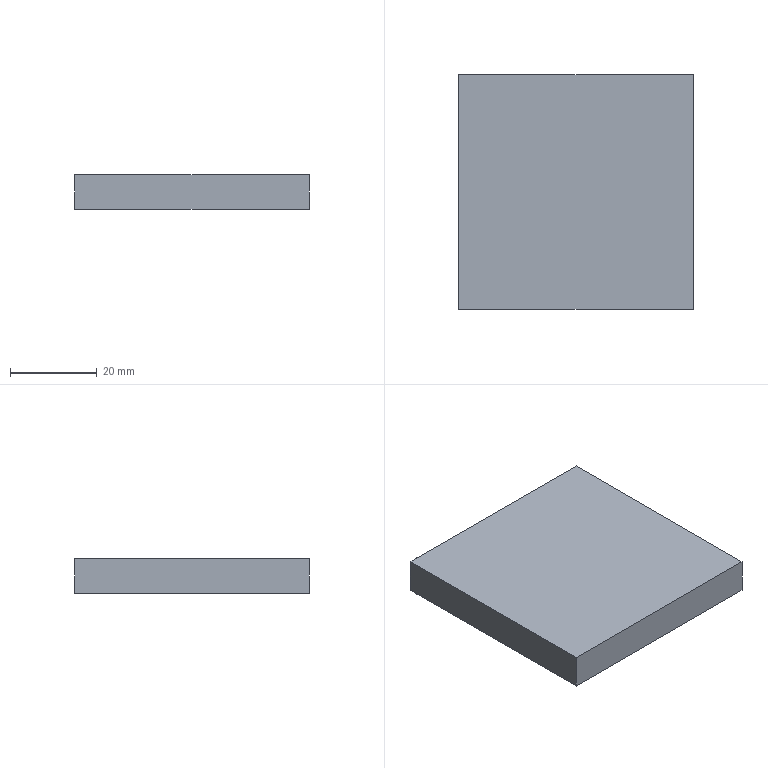Part | STEP file | X77-03113 | 1 solid | 6 faces | box 54 x 54 x 8 mm | volume 23328 mm3 | plane 6
STEP:
#1=CARTESIAN_POINT('',(3257.,-3.,0.));
#2=VERTEX_POINT('',#1);
#3=CARTESIAN_POINT('',(3203.,-3.,0.));
#4=VERTEX_POINT('',#3);
#5=CARTESIAN_POINT('',(3257.,-3.,0.));
#6=DIRECTION('',(-1.,0.,0.));
#7=VECTOR('',#6,1000.);
#8=LINE('',#5,#7);
#9=EDGE_CURVE('',#2,#4,#8,.T.);
#10=ORIENTED_EDGE('',*,*,#9,.F.);
#11=CARTESIAN_POINT('',(3257.,-3.,-8.));
#12=VERTEX_POINT('',#11);
#13=CARTESIAN_POINT('',(3257.,-3.,-8.));
#14=DIRECTION('',(0.,0.,1.));
#15=VECTOR('',#14,1000.);
#16=LINE('',#13,#15);
#17=EDGE_CURVE('',#12,#2,#16,.T.);
#18=ORIENTED_EDGE('',*,*,#17,.F.);
#19=CARTESIAN_POINT('',(3203.,-3.,-8.));
#20=VERTEX_POINT('',#19);
#21=CARTESIAN_POINT('',(3257.,-3.,-8.));
#22=DIRECTION('',(-1.,0.,0.));
#23=VECTOR('',#22,1000.);
#24=LINE('',#21,#23);
#25=EDGE_CURVE('',#12,#20,#24,.T.);
#26=ORIENTED_EDGE('',*,*,#25,.T.);
#27=CARTESIAN_POINT('',(3203.,-3.,-8.));
#28=DIRECTION('',(0.,0.,1.));
#29=VECTOR('',#28,1000.);
#30=LINE('',#27,#29);
#31=EDGE_CURVE('',#20,#4,#30,.T.);
#32=ORIENTED_EDGE('',*,*,#31,.T.);
#33=EDGE_LOOP('',(#10,#18,#26,#32));
#34=FACE_OUTER_BOUND('',#33,.T.);
#35=CARTESIAN_POINT('',(3257.,-3.,-8.));
#36=DIRECTION('',(0.,1.,0.));
#37=DIRECTION('',(-1.,0.,0.));
#38=AXIS2_PLACEMENT_3D('',#35,#36,#37);
#39=PLANE('',#38);
#40=ADVANCED_FACE('',(#34),#39,.T.);
#41=CARTESIAN_POINT('',(3257.,-57.,0.));
#42=VERTEX_POINT('',#41);
#43=CARTESIAN_POINT('',(3257.,-3.,0.));
#44=DIRECTION('',(0.,1.,0.));
#45=VECTOR('',#44,1000.);
#46=LINE('',#43,#45);
#47=EDGE_CURVE('',#42,#2,#46,.T.);
#48=ORIENTED_EDGE('',*,*,#47,.F.);
#49=CARTESIAN_POINT('',(3257.,-57.,-8.));
#50=VERTEX_POINT('',#49);
#51=CARTESIAN_POINT('',(3257.,-57.,-8.));
#52=DIRECTION('',(0.,0.,1.));
#53=VECTOR('',#52,1000.);
#54=LINE('',#51,#53);
#55=EDGE_CURVE('',#50,#42,#54,.T.);
#56=ORIENTED_EDGE('',*,*,#55,.F.);
#57=CARTESIAN_POINT('',(3257.,-3.,-8.));
#58=DIRECTION('',(0.,1.,0.));
#59=VECTOR('',#58,1000.);
#60=LINE('',#57,#59);
#61=EDGE_CURVE('',#50,#12,#60,.T.);
#62=ORIENTED_EDGE('',*,*,#61,.T.);
#63=ORIENTED_EDGE('',*,*,#17,.T.);
#64=EDGE_LOOP('',(#48,#56,#62,#63));
#65=FACE_OUTER_BOUND('',#64,.T.);
#66=CARTESIAN_POINT('',(3257.,-3.,-8.));
#67=DIRECTION('',(1.,0.,0.));
#68=DIRECTION('',(0.,0.,-1.));
#69=AXIS2_PLACEMENT_3D('',#66,#67,#68);
#70=PLANE('',#69);
#71=ADVANCED_FACE('',(#65),#70,.T.);
#72=CARTESIAN_POINT('',(3203.,-57.,0.));
#73=VERTEX_POINT('',#72);
#74=CARTESIAN_POINT('',(3257.,-57.,0.));
#75=DIRECTION('',(1.,0.,0.));
#76=VECTOR('',#75,1000.);
#77=LINE('',#74,#76);
#78=EDGE_CURVE('',#73,#42,#77,.T.);
#79=ORIENTED_EDGE('',*,*,#78,.F.);
#80=CARTESIAN_POINT('',(3203.,-57.,-8.));
#81=VERTEX_POINT('',#80);
#82=CARTESIAN_POINT('',(3203.,-57.,-8.));
#83=DIRECTION('',(0.,0.,1.));
#84=VECTOR('',#83,1000.);
#85=LINE('',#82,#84);
#86=EDGE_CURVE('',#81,#73,#85,.T.);
#87=ORIENTED_EDGE('',*,*,#86,.F.);
#88=CARTESIAN_POINT('',(3257.,-57.,-8.));
#89=DIRECTION('',(1.,0.,0.));
#90=VECTOR('',#89,1000.);
#91=LINE('',#88,#90);
#92=EDGE_CURVE('',#81,#50,#91,.T.);
#93=ORIENTED_EDGE('',*,*,#92,.T.);
#94=ORIENTED_EDGE('',*,*,#55,.T.);
#95=EDGE_LOOP('',(#79,#87,#93,#94));
#96=FACE_OUTER_BOUND('',#95,.T.);
#97=CARTESIAN_POINT('',(3257.,-57.,-8.));
#98=DIRECTION('',(0.,-1.,0.));
#99=DIRECTION('',(1.,0.,0.));
#100=AXIS2_PLACEMENT_3D('',#97,#98,#99);
#101=PLANE('',#100);
#102=ADVANCED_FACE('',(#96),#101,.T.);
#103=CARTESIAN_POINT('',(3203.,-57.,0.));
#104=DIRECTION('',(0.,-1.,0.));
#105=VECTOR('',#104,1000.);
#106=LINE('',#103,#105);
#107=EDGE_CURVE('',#4,#73,#106,.T.);
#108=ORIENTED_EDGE('',*,*,#107,.F.);
#109=ORIENTED_EDGE('',*,*,#31,.F.);
#110=CARTESIAN_POINT('',(3203.,-57.,-8.));
#111=DIRECTION('',(0.,-1.,0.));
#112=VECTOR('',#111,1000.);
#113=LINE('',#110,#112);
#114=EDGE_CURVE('',#20,#81,#113,.T.);
#115=ORIENTED_EDGE('',*,*,#114,.T.);
#116=ORIENTED_EDGE('',*,*,#86,.T.);
#117=EDGE_LOOP('',(#108,#109,#115,#116));
#118=FACE_OUTER_BOUND('',#117,.T.);
#119=CARTESIAN_POINT('',(3203.,-57.,-8.));
#120=DIRECTION('',(-1.,0.,0.));
#121=DIRECTION('',(0.,0.,1.));
#122=AXIS2_PLACEMENT_3D('',#119,#120,#121);
#123=PLANE('',#122);
#124=ADVANCED_FACE('',(#118),#123,.T.);
#125=ORIENTED_EDGE('',*,*,#25,.F.);
#126=ORIENTED_EDGE('',*,*,#61,.F.);
#127=ORIENTED_EDGE('',*,*,#92,.F.);
#128=ORIENTED_EDGE('',*,*,#114,.F.);
#129=EDGE_LOOP('',(#125,#126,#127,#128));
#130=FACE_OUTER_BOUND('',#129,.T.);
#131=CARTESIAN_POINT('',(3203.,-3.,-8.));
#132=DIRECTION('',(0.,0.,-1.));
#133=DIRECTION('',(-1.,0.,0.));
#134=AXIS2_PLACEMENT_3D('',#131,#132,#133);
#135=PLANE('',#134);
#136=ADVANCED_FACE('',(#130),#135,.T.);
#137=ORIENTED_EDGE('',*,*,#9,.T.);
#138=ORIENTED_EDGE('',*,*,#107,.T.);
#139=ORIENTED_EDGE('',*,*,#78,.T.);
#140=ORIENTED_EDGE('',*,*,#47,.T.);
#141=EDGE_LOOP('',(#137,#138,#139,#140));
#142=FACE_OUTER_BOUND('',#141,.T.);
#143=CARTESIAN_POINT('',(3203.,-3.,0.));
#144=DIRECTION('',(0.,0.,-1.));
#145=DIRECTION('',(-1.,0.,0.));
#146=AXIS2_PLACEMENT_3D('',#143,#144,#145);
#147=PLANE('',#146);
#148=ADVANCED_FACE('',(#142),#147,.F.);
#149=CLOSED_SHELL('',(#40,#71,#102,#124,#136,#148));
#150=MANIFOLD_SOLID_BREP('',#149);
#151=CARTESIAN_POINT('',(0.,0.,0.));
#152=DIRECTION('',(0.,0.,1.));
#153=DIRECTION('',(1.,0.,0.));
#154=AXIS2_PLACEMENT_3D('',#151,#152,#153);
#155=(LENGTH_UNIT()NAMED_UNIT(*)SI_UNIT(.MILLI.,.METRE.));
#156=UNCERTAINTY_MEASURE_WITH_UNIT(LENGTH_MEASURE(0.00001),#155,'','');
#157=(NAMED_UNIT(*)PLANE_ANGLE_UNIT()SI_UNIT($,.RADIAN.));
#158=(NAMED_UNIT(*)SI_UNIT($,.STERADIAN.)SOLID_ANGLE_UNIT());
#159=(GEOMETRIC_REPRESENTATION_CONTEXT(3)GLOBAL_UNCERTAINTY_ASSIGNED_CONTEXT((#156))GLOBAL_UNIT_ASSIGNED_CONTEXT((#155,#157,#158))REPRESENTATION_CONTEXT('',''));
#160=ADVANCED_BREP_SHAPE_REPRESENTATION('',(#150,#154),#159);